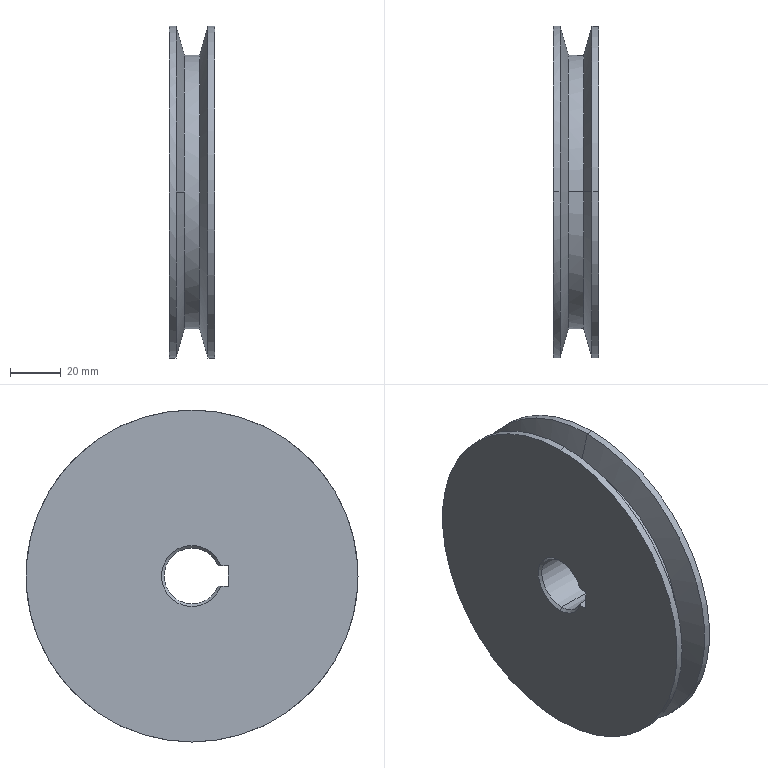Part | SolidWorks | features BaseBody 1 | 1 solid | 24 faces | box 18 x 130.5 x 130.5 mm | volume 193093 mm3 | cone 10 | cylinder 9 | plane 5 | commonest cylinder face diameters 130.5 x4 22 x3 107.6 x2
STEP:
#1=CARTESIAN_POINT('',(18.,0.,65.25));
#2=VERTEX_POINT('',#1);
#3=CARTESIAN_POINT('',(18.,0.,-65.25));
#4=VERTEX_POINT('',#3);
#5=CARTESIAN_POINT('',(18.,0.,0.));
#6=DIRECTION('',(-1.,0.,0.));
#7=DIRECTION('',(0.,0.,1.));
#8=AXIS2_PLACEMENT_3D('',#5,#6,#7);
#9=CIRCLE('',#8,65.25);
#10=EDGE_CURVE('',#2,#4,#9,.T.);
#11=ORIENTED_EDGE('',*,*,#10,.T.);
#12=CARTESIAN_POINT('',(15.289,0.,-65.25));
#13=VERTEX_POINT('',#12);
#14=CARTESIAN_POINT('',(0.,0.,-65.25));
#15=DIRECTION('',(-1.,0.,0.));
#16=VECTOR('',#15,1000.);
#17=LINE('',#14,#16);
#18=EDGE_CURVE('',#4,#13,#17,.T.);
#19=ORIENTED_EDGE('',*,*,#18,.T.);
#20=CARTESIAN_POINT('',(15.289,0.,65.25));
#21=VERTEX_POINT('',#20);
#22=CARTESIAN_POINT('',(15.289,0.,0.));
#23=DIRECTION('',(1.,0.,0.));
#24=DIRECTION('',(0.,0.,1.));
#25=AXIS2_PLACEMENT_3D('',#22,#23,#24);
#26=CIRCLE('',#25,65.25);
#27=EDGE_CURVE('',#13,#21,#26,.T.);
#28=ORIENTED_EDGE('',*,*,#27,.T.);
#29=CARTESIAN_POINT('',(0.,0.,65.25));
#30=DIRECTION('',(-1.,0.,0.));
#31=VECTOR('',#30,1000.);
#32=LINE('',#29,#31);
#33=EDGE_CURVE('',#2,#21,#32,.T.);
#34=ORIENTED_EDGE('',*,*,#33,.F.);
#35=EDGE_LOOP('',(#11,#19,#28,#34));
#36=FACE_OUTER_BOUND('',#35,.T.);
#37=CARTESIAN_POINT('',(0.,0.,0.));
#38=DIRECTION('',(-1.,0.,0.));
#39=DIRECTION('',(0.,0.,1.));
#40=AXIS2_PLACEMENT_3D('',#37,#38,#39);
#41=CYLINDRICAL_SURFACE('',#40,65.25);
#42=ADVANCED_FACE('',(#36),#41,.T.);
#43=CARTESIAN_POINT('',(17.,0.,11.));
#44=VERTEX_POINT('',#43);
#45=CARTESIAN_POINT('',(17.,-10.247,4.));
#46=VERTEX_POINT('',#45);
#47=CARTESIAN_POINT('',(17.,0.,0.));
#48=DIRECTION('',(1.,0.,0.));
#49=DIRECTION('',(0.,0.,-1.));
#50=AXIS2_PLACEMENT_3D('',#47,#48,#49);
#51=CIRCLE('',#50,11.);
#52=EDGE_CURVE('',#44,#46,#51,.T.);
#53=ORIENTED_EDGE('',*,*,#52,.F.);
#54=CARTESIAN_POINT('',(18.,0.,12.));
#55=VERTEX_POINT('',#54);
#56=CARTESIAN_POINT('',(18.,0.,12.));
#57=DIRECTION('',(0.7071,0.,0.7071));
#58=VECTOR('',#57,1000.);
#59=LINE('',#56,#58);
#60=EDGE_CURVE('',#44,#55,#59,.T.);
#61=ORIENTED_EDGE('',*,*,#60,.T.);
#62=CARTESIAN_POINT('',(18.,-11.314,4.));
#63=VERTEX_POINT('',#62);
#64=CARTESIAN_POINT('',(18.,0.,0.));
#65=DIRECTION('',(1.,0.,0.));
#66=DIRECTION('',(0.,0.,-1.));
#67=AXIS2_PLACEMENT_3D('',#64,#65,#66);
#68=CIRCLE('',#67,12.);
#69=EDGE_CURVE('',#55,#63,#68,.T.);
#70=ORIENTED_EDGE('',*,*,#69,.T.);
#71=CARTESIAN_POINT('',(18.,-11.314,4.));
#72=CARTESIAN_POINT('',(17.666,-10.959,4.));
#73=CARTESIAN_POINT('',(17.332,-10.604,4.));
#74=CARTESIAN_POINT('',(17.,-10.247,4.));
#75=B_SPLINE_CURVE_WITH_KNOTS('',3,(#71,#72,#73,#74),.UNSPECIFIED.,.F.,.F.,(4,4),(0.,0.001462),.UNSPECIFIED.);
#76=EDGE_CURVE('',#63,#46,#75,.T.);
#77=ORIENTED_EDGE('',*,*,#76,.T.);
#78=EDGE_LOOP('',(#53,#61,#70,#77));
#79=FACE_OUTER_BOUND('',#78,.T.);
#80=CARTESIAN_POINT('',(18.,0.,0.));
#81=DIRECTION('',(1.,0.,0.));
#82=DIRECTION('',(0.,0.,-1.));
#83=AXIS2_PLACEMENT_3D('',#80,#81,#82);
#84=CONICAL_SURFACE('',#83,12.,0.7854);
#85=ADVANCED_FACE('',(#79),#84,.F.);
#86=ORIENTED_EDGE('',*,*,#60,.F.);
#87=CARTESIAN_POINT('',(17.,0.,-11.));
#88=VERTEX_POINT('',#87);
#89=CARTESIAN_POINT('',(17.,0.,0.));
#90=DIRECTION('',(1.,0.,0.));
#91=DIRECTION('',(0.,0.,-1.));
#92=AXIS2_PLACEMENT_3D('',#89,#90,#91);
#93=CIRCLE('',#92,11.);
#94=EDGE_CURVE('',#88,#44,#93,.T.);
#95=ORIENTED_EDGE('',*,*,#94,.F.);
#96=CARTESIAN_POINT('',(18.,0.,-12.));
#97=VERTEX_POINT('',#96);
#98=CARTESIAN_POINT('',(18.,0.,-12.));
#99=DIRECTION('',(0.7071,0.,-0.7071));
#100=VECTOR('',#99,1000.);
#101=LINE('',#98,#100);
#102=EDGE_CURVE('',#88,#97,#101,.T.);
#103=ORIENTED_EDGE('',*,*,#102,.T.);
#104=CARTESIAN_POINT('',(18.,0.,0.));
#105=DIRECTION('',(1.,0.,0.));
#106=DIRECTION('',(0.,0.,-1.));
#107=AXIS2_PLACEMENT_3D('',#104,#105,#106);
#108=CIRCLE('',#107,12.);
#109=EDGE_CURVE('',#97,#55,#108,.T.);
#110=ORIENTED_EDGE('',*,*,#109,.T.);
#111=EDGE_LOOP('',(#86,#95,#103,#110));
#112=FACE_OUTER_BOUND('',#111,.T.);
#113=CARTESIAN_POINT('',(18.,0.,0.));
#114=DIRECTION('',(1.,0.,0.));
#115=DIRECTION('',(0.,0.,-1.));
#116=AXIS2_PLACEMENT_3D('',#113,#114,#115);
#117=CONICAL_SURFACE('',#116,12.,0.7854);
#118=ADVANCED_FACE('',(#112),#117,.F.);
#119=CARTESIAN_POINT('',(12.005,0.,-53.8));
#120=VERTEX_POINT('',#119);
#121=CARTESIAN_POINT('',(12.005,0.,53.8));
#122=VERTEX_POINT('',#121);
#123=CARTESIAN_POINT('',(12.005,0.,0.));
#124=DIRECTION('',(1.,0.,0.));
#125=DIRECTION('',(0.,0.,-1.));
#126=AXIS2_PLACEMENT_3D('',#123,#124,#125);
#127=CIRCLE('',#126,53.8);
#128=EDGE_CURVE('',#120,#122,#127,.T.);
#129=ORIENTED_EDGE('',*,*,#128,.T.);
#130=CARTESIAN_POINT('',(15.289,0.,65.25));
#131=DIRECTION('',(0.2756,0.,0.9613));
#132=VECTOR('',#131,1000.);
#133=LINE('',#130,#132);
#134=EDGE_CURVE('',#122,#21,#133,.T.);
#135=ORIENTED_EDGE('',*,*,#134,.T.);
#136=ORIENTED_EDGE('',*,*,#27,.F.);
#137=CARTESIAN_POINT('',(15.289,0.,-65.25));
#138=DIRECTION('',(0.2756,0.,-0.9613));
#139=VECTOR('',#138,1000.);
#140=LINE('',#137,#139);
#141=EDGE_CURVE('',#120,#13,#140,.T.);
#142=ORIENTED_EDGE('',*,*,#141,.F.);
#143=EDGE_LOOP('',(#129,#135,#136,#142));
#144=FACE_OUTER_BOUND('',#143,.T.);
#145=CARTESIAN_POINT('',(15.289,0.,0.));
#146=DIRECTION('',(1.,0.,0.));
#147=DIRECTION('',(0.,0.,-1.));
#148=AXIS2_PLACEMENT_3D('',#145,#146,#147);
#149=CONICAL_SURFACE('',#148,65.25,1.292);
#150=ADVANCED_FACE('',(#144),#149,.T.);
#151=CARTESIAN_POINT('',(17.,-10.247,-4.));
#152=VERTEX_POINT('',#151);
#153=CARTESIAN_POINT('',(17.,0.,0.));
#154=DIRECTION('',(1.,0.,0.));
#155=DIRECTION('',(0.,0.,-1.));
#156=AXIS2_PLACEMENT_3D('',#153,#154,#155);
#157=CIRCLE('',#156,11.);
#158=EDGE_CURVE('',#152,#88,#157,.T.);
#159=ORIENTED_EDGE('',*,*,#158,.T.);
#160=CARTESIAN_POINT('',(1.,0.,-11.));
#161=VERTEX_POINT('',#160);
#162=CARTESIAN_POINT('',(0.,0.,-11.));
#163=DIRECTION('',(-1.,0.,0.));
#164=VECTOR('',#163,1000.);
#165=LINE('',#162,#164);
#166=EDGE_CURVE('',#88,#161,#165,.T.);
#167=ORIENTED_EDGE('',*,*,#166,.T.);
#168=CARTESIAN_POINT('',(1.,-10.247,-4.));
#169=VERTEX_POINT('',#168);
#170=CARTESIAN_POINT('',(1.,0.,0.));
#171=DIRECTION('',(1.,0.,0.));
#172=DIRECTION('',(0.,0.,1.));
#173=AXIS2_PLACEMENT_3D('',#170,#171,#172);
#174=CIRCLE('',#173,11.);
#175=EDGE_CURVE('',#169,#161,#174,.T.);
#176=ORIENTED_EDGE('',*,*,#175,.F.);
#177=CARTESIAN_POINT('',(44.,-10.247,-4.));
#178=DIRECTION('',(1.,0.,0.));
#179=VECTOR('',#178,1000.);
#180=LINE('',#177,#179);
#181=EDGE_CURVE('',#169,#152,#180,.T.);
#182=ORIENTED_EDGE('',*,*,#181,.T.);
#183=EDGE_LOOP('',(#159,#167,#176,#182));
#184=FACE_OUTER_BOUND('',#183,.T.);
#185=CARTESIAN_POINT('',(0.,0.,0.));
#186=DIRECTION('',(-1.,0.,0.));
#187=DIRECTION('',(0.,0.,1.));
#188=AXIS2_PLACEMENT_3D('',#185,#186,#187);
#189=CYLINDRICAL_SURFACE('',#188,11.);
#190=ADVANCED_FACE('',(#184),#189,.F.);
#191=ORIENTED_EDGE('',*,*,#166,.F.);
#192=ORIENTED_EDGE('',*,*,#94,.T.);
#193=CARTESIAN_POINT('',(1.,0.,11.));
#194=VERTEX_POINT('',#193);
#195=CARTESIAN_POINT('',(0.,0.,11.));
#196=DIRECTION('',(-1.,0.,0.));
#197=VECTOR('',#196,1000.);
#198=LINE('',#195,#197);
#199=EDGE_CURVE('',#44,#194,#198,.T.);
#200=ORIENTED_EDGE('',*,*,#199,.T.);
#201=CARTESIAN_POINT('',(1.,0.,0.));
#202=DIRECTION('',(1.,0.,0.));
#203=DIRECTION('',(0.,0.,1.));
#204=AXIS2_PLACEMENT_3D('',#201,#202,#203);
#205=CIRCLE('',#204,11.);
#206=EDGE_CURVE('',#161,#194,#205,.T.);
#207=ORIENTED_EDGE('',*,*,#206,.F.);
#208=EDGE_LOOP('',(#191,#192,#200,#207));
#209=FACE_OUTER_BOUND('',#208,.T.);
#210=CARTESIAN_POINT('',(0.,0.,0.));
#211=DIRECTION('',(-1.,0.,0.));
#212=DIRECTION('',(0.,0.,1.));
#213=AXIS2_PLACEMENT_3D('',#210,#211,#212);
#214=CYLINDRICAL_SURFACE('',#213,11.);
#215=ADVANCED_FACE('',(#209),#214,.F.);
#216=ORIENTED_EDGE('',*,*,#128,.F.);
#217=CARTESIAN_POINT('',(5.995,0.,-53.8));
#218=VERTEX_POINT('',#217);
#219=CARTESIAN_POINT('',(0.,0.,-53.8));
#220=DIRECTION('',(-1.,0.,0.));
#221=VECTOR('',#220,1000.);
#222=LINE('',#219,#221);
#223=EDGE_CURVE('',#120,#218,#222,.T.);
#224=ORIENTED_EDGE('',*,*,#223,.T.);
#225=CARTESIAN_POINT('',(5.995,53.8,0.));
#226=VERTEX_POINT('',#225);
#227=CARTESIAN_POINT('',(5.995,0.,0.));
#228=DIRECTION('',(1.,0.,0.));
#229=DIRECTION('',(0.,0.,1.));
#230=AXIS2_PLACEMENT_3D('',#227,#228,#229);
#231=CIRCLE('',#230,53.8);
#232=EDGE_CURVE('',#218,#226,#231,.T.);
#233=ORIENTED_EDGE('',*,*,#232,.T.);
#234=CARTESIAN_POINT('',(5.995,0.,53.8));
#235=VERTEX_POINT('',#234);
#236=CARTESIAN_POINT('',(5.995,0.,0.));
#237=DIRECTION('',(1.,0.,0.));
#238=DIRECTION('',(0.,0.,1.));
#239=AXIS2_PLACEMENT_3D('',#236,#237,#238);
#240=CIRCLE('',#239,53.8);
#241=EDGE_CURVE('',#226,#235,#240,.T.);
#242=ORIENTED_EDGE('',*,*,#241,.T.);
#243=CARTESIAN_POINT('',(0.,0.,53.8));
#244=DIRECTION('',(-1.,0.,0.));
#245=VECTOR('',#244,1000.);
#246=LINE('',#243,#245);
#247=EDGE_CURVE('',#122,#235,#246,.T.);
#248=ORIENTED_EDGE('',*,*,#247,.F.);
#249=EDGE_LOOP('',(#216,#224,#233,#242,#248));
#250=FACE_OUTER_BOUND('',#249,.T.);
#251=CARTESIAN_POINT('',(0.,0.,0.));
#252=DIRECTION('',(-1.,0.,0.));
#253=DIRECTION('',(0.,0.,1.));
#254=AXIS2_PLACEMENT_3D('',#251,#252,#253);
#255=CYLINDRICAL_SURFACE('',#254,53.8);
#256=ADVANCED_FACE('',(#250),#255,.T.);
#257=CARTESIAN_POINT('',(2.711,65.25,0.));
#258=VERTEX_POINT('',#257);
#259=CARTESIAN_POINT('',(2.711,0.,-65.25));
#260=VERTEX_POINT('',#259);
#261=CARTESIAN_POINT('',(2.711,0.,0.));
#262=DIRECTION('',(-1.,0.,0.));
#263=DIRECTION('',(0.,0.,1.));
#264=AXIS2_PLACEMENT_3D('',#261,#262,#263);
#265=CIRCLE('',#264,65.25);
#266=EDGE_CURVE('',#258,#260,#265,.T.);
#267=ORIENTED_EDGE('',*,*,#266,.T.);
#268=CARTESIAN_POINT('',(0.,0.,-65.25));
#269=VERTEX_POINT('',#268);
#270=CARTESIAN_POINT('',(0.,0.,-65.25));
#271=DIRECTION('',(-1.,0.,0.));
#272=VECTOR('',#271,1000.);
#273=LINE('',#270,#272);
#274=EDGE_CURVE('',#260,#269,#273,.T.);
#275=ORIENTED_EDGE('',*,*,#274,.T.);
#276=CARTESIAN_POINT('',(0.,0.,65.25));
#277=VERTEX_POINT('',#276);
#278=CARTESIAN_POINT('',(0.,0.,0.));
#279=DIRECTION('',(1.,0.,0.));
#280=DIRECTION('',(0.,0.,1.));
#281=AXIS2_PLACEMENT_3D('',#278,#279,#280);
#282=CIRCLE('',#281,65.25);
#283=EDGE_CURVE('',#269,#277,#282,.T.);
#284=ORIENTED_EDGE('',*,*,#283,.T.);
#285=CARTESIAN_POINT('',(2.711,0.,65.25));
#286=VERTEX_POINT('',#285);
#287=CARTESIAN_POINT('',(0.,0.,65.25));
#288=DIRECTION('',(-1.,0.,0.));
#289=VECTOR('',#288,1000.);
#290=LINE('',#287,#289);
#291=EDGE_CURVE('',#286,#277,#290,.T.);
#292=ORIENTED_EDGE('',*,*,#291,.F.);
#293=CARTESIAN_POINT('',(2.711,0.,0.));
#294=DIRECTION('',(-1.,0.,0.));
#295=DIRECTION('',(0.,0.,1.));
#296=AXIS2_PLACEMENT_3D('',#293,#294,#295);
#297=CIRCLE('',#296,65.25);
#298=EDGE_CURVE('',#286,#258,#297,.T.);
#299=ORIENTED_EDGE('',*,*,#298,.T.);
#300=EDGE_LOOP('',(#267,#275,#284,#292,#299));
#301=FACE_OUTER_BOUND('',#300,.T.);
#302=CARTESIAN_POINT('',(0.,0.,0.));
#303=DIRECTION('',(-1.,0.,0.));
#304=DIRECTION('',(0.,0.,1.));
#305=AXIS2_PLACEMENT_3D('',#302,#303,#304);
#306=CYLINDRICAL_SURFACE('',#305,65.25);
#307=ADVANCED_FACE('',(#301),#306,.T.);
#308=ORIENTED_EDGE('',*,*,#175,.T.);
#309=CARTESIAN_POINT('',(0.,0.,-12.));
#310=VERTEX_POINT('',#309);
#311=CARTESIAN_POINT('',(0.,0.,-12.));
#312=DIRECTION('',(-0.7071,0.,-0.7071));
#313=VECTOR('',#312,1000.);
#314=LINE('',#311,#313);
#315=EDGE_CURVE('',#161,#310,#314,.T.);
#316=ORIENTED_EDGE('',*,*,#315,.T.);
#317=CARTESIAN_POINT('',(0.,-11.314,-4.));
#318=VERTEX_POINT('',#317);
#319=CARTESIAN_POINT('',(0.,0.,0.));
#320=DIRECTION('',(-1.,0.,0.));
#321=DIRECTION('',(0.,0.,1.));
#322=AXIS2_PLACEMENT_3D('',#319,#320,#321);
#323=CIRCLE('',#322,12.);
#324=EDGE_CURVE('',#310,#318,#323,.T.);
#325=ORIENTED_EDGE('',*,*,#324,.T.);
#326=CARTESIAN_POINT('',(1.,-10.247,-4.));
#327=CARTESIAN_POINT('',(0.6832,-10.587,-4.));
#328=CARTESIAN_POINT('',(0.3498,-10.943,-4.));
#329=CARTESIAN_POINT('',(0.,-11.314,-4.));
#330=B_SPLINE_CURVE_WITH_KNOTS('',3,(#326,#327,#328,#329),.UNSPECIFIED.,.F.,.F.,(4,4),(0.,1.),.UNSPECIFIED.);
#331=EDGE_CURVE('',#169,#318,#330,.T.);
#332=ORIENTED_EDGE('',*,*,#331,.F.);
#333=EDGE_LOOP('',(#308,#316,#325,#332));
#334=FACE_OUTER_BOUND('',#333,.T.);
#335=CARTESIAN_POINT('',(0.,0.,0.));
#336=DIRECTION('',(-1.,0.,0.));
#337=DIRECTION('',(0.,0.,1.));
#338=AXIS2_PLACEMENT_3D('',#335,#336,#337);
#339=CONICAL_SURFACE('',#338,12.,0.7854);
#340=ADVANCED_FACE('',(#334),#339,.F.);
#341=ORIENTED_EDGE('',*,*,#315,.F.);
#342=ORIENTED_EDGE('',*,*,#206,.T.);
#343=CARTESIAN_POINT('',(0.,0.,12.));
#344=VERTEX_POINT('',#343);
#345=CARTESIAN_POINT('',(0.,0.,12.));
#346=DIRECTION('',(-0.7071,0.,0.7071));
#347=VECTOR('',#346,1000.);
#348=LINE('',#345,#347);
#349=EDGE_CURVE('',#194,#344,#348,.T.);
#350=ORIENTED_EDGE('',*,*,#349,.T.);
#351=CARTESIAN_POINT('',(0.,0.,0.));
#352=DIRECTION('',(-1.,0.,0.));
#353=DIRECTION('',(0.,0.,1.));
#354=AXIS2_PLACEMENT_3D('',#351,#352,#353);
#355=CIRCLE('',#354,12.);
#356=EDGE_CURVE('',#344,#310,#355,.T.);
#357=ORIENTED_EDGE('',*,*,#356,.T.);
#358=EDGE_LOOP('',(#341,#342,#350,#357));
#359=FACE_OUTER_BOUND('',#358,.T.);
#360=CARTESIAN_POINT('',(0.,0.,0.));
#361=DIRECTION('',(-1.,0.,0.));
#362=DIRECTION('',(0.,0.,1.));
#363=AXIS2_PLACEMENT_3D('',#360,#361,#362);
#364=CONICAL_SURFACE('',#363,12.,0.7854);
#365=ADVANCED_FACE('',(#359),#364,.F.);
#366=ORIENTED_EDGE('',*,*,#241,.F.);
#367=CARTESIAN_POINT('',(2.711,65.25,0.));
#368=DIRECTION('',(-0.2756,0.9613,0.));
#369=VECTOR('',#368,1000.);
#370=LINE('',#367,#369);
#371=EDGE_CURVE('',#226,#258,#370,.T.);
#372=ORIENTED_EDGE('',*,*,#371,.T.);
#373=ORIENTED_EDGE('',*,*,#298,.F.);
#374=CARTESIAN_POINT('',(2.711,-65.25,0.));
#375=VERTEX_POINT('',#374);
#376=CARTESIAN_POINT('',(2.711,0.,0.));
#377=DIRECTION('',(-1.,0.,0.));
#378=DIRECTION('',(0.,0.,1.));
#379=AXIS2_PLACEMENT_3D('',#376,#377,#378);
#380=CIRCLE('',#379,65.25);
#381=EDGE_CURVE('',#375,#286,#380,.T.);
#382=ORIENTED_EDGE('',*,*,#381,.F.);
#383=CARTESIAN_POINT('',(5.995,-53.8,0.));
#384=VERTEX_POINT('',#383);
#385=CARTESIAN_POINT('',(2.711,-65.25,0.));
#386=DIRECTION('',(-0.2756,-0.9613,0.));
#387=VECTOR('',#386,1000.);
#388=LINE('',#385,#387);
#389=EDGE_CURVE('',#384,#375,#388,.T.);
#390=ORIENTED_EDGE('',*,*,#389,.F.);
#391=CARTESIAN_POINT('',(5.995,0.,0.));
#392=DIRECTION('',(1.,0.,0.));
#393=DIRECTION('',(0.,0.,1.));
#394=AXIS2_PLACEMENT_3D('',#391,#392,#393);
#395=CIRCLE('',#394,53.8);
#396=EDGE_CURVE('',#235,#384,#395,.T.);
#397=ORIENTED_EDGE('',*,*,#396,.F.);
#398=EDGE_LOOP('',(#366,#372,#373,#382,#390,#397));
#399=FACE_OUTER_BOUND('',#398,.T.);
#400=CARTESIAN_POINT('',(2.711,0.,0.));
#401=DIRECTION('',(-1.,0.,0.));
#402=DIRECTION('',(0.,-1.,0.));
#403=AXIS2_PLACEMENT_3D('',#400,#401,#402);
#404=CONICAL_SURFACE('',#403,65.25,1.292);
#405=ADVANCED_FACE('',(#399),#404,.T.);
#406=ORIENTED_EDGE('',*,*,#10,.F.);
#407=CARTESIAN_POINT('',(18.,0.,0.));
#408=DIRECTION('',(-1.,0.,0.));
#409=DIRECTION('',(0.,0.,1.));
#410=AXIS2_PLACEMENT_3D('',#407,#408,#409);
#411=CIRCLE('',#410,65.25);
#412=EDGE_CURVE('',#4,#2,#411,.T.);
#413=ORIENTED_EDGE('',*,*,#412,.F.);
#414=EDGE_LOOP('',(#406,#413));
#415=FACE_OUTER_BOUND('',#414,.T.);
#416=CARTESIAN_POINT('',(18.,-14.3,4.));
#417=VERTEX_POINT('',#416);
#418=CARTESIAN_POINT('',(18.,65.25,4.));
#419=DIRECTION('',(0.,-1.,0.));
#420=VECTOR('',#419,1000.);
#421=LINE('',#418,#420);
#422=EDGE_CURVE('',#63,#417,#421,.T.);
#423=ORIENTED_EDGE('',*,*,#422,.F.);
#424=ORIENTED_EDGE('',*,*,#69,.F.);
#425=ORIENTED_EDGE('',*,*,#109,.F.);
#426=CARTESIAN_POINT('',(18.,-11.314,-4.));
#427=VERTEX_POINT('',#426);
#428=CARTESIAN_POINT('',(18.,0.,0.));
#429=DIRECTION('',(1.,0.,0.));
#430=DIRECTION('',(0.,0.,-1.));
#431=AXIS2_PLACEMENT_3D('',#428,#429,#430);
#432=CIRCLE('',#431,12.);
#433=EDGE_CURVE('',#427,#97,#432,.T.);
#434=ORIENTED_EDGE('',*,*,#433,.F.);
#435=CARTESIAN_POINT('',(18.,-14.3,-4.));
#436=VERTEX_POINT('',#435);
#437=CARTESIAN_POINT('',(18.,65.25,-4.));
#438=DIRECTION('',(0.,1.,0.));
#439=VECTOR('',#438,1000.);
#440=LINE('',#437,#439);
#441=EDGE_CURVE('',#436,#427,#440,.T.);
#442=ORIENTED_EDGE('',*,*,#441,.F.);
#443=CARTESIAN_POINT('',(18.,-14.3,0.));
#444=DIRECTION('',(0.,0.,-1.));
#445=VECTOR('',#444,1000.);
#446=LINE('',#443,#445);
#447=EDGE_CURVE('',#417,#436,#446,.T.);
#448=ORIENTED_EDGE('',*,*,#447,.F.);
#449=EDGE_LOOP('',(#423,#424,#425,#434,#442,#448));
#450=FACE_BOUND('',#449,.T.);
#451=CARTESIAN_POINT('',(18.,65.25,0.));
#452=DIRECTION('',(-1.,0.,0.));
#453=DIRECTION('',(0.,0.,1.));
#454=AXIS2_PLACEMENT_3D('',#451,#452,#453);
#455=PLANE('',#454);
#456=ADVANCED_FACE('',(#415,#450),#455,.F.);
#457=ORIENTED_EDGE('',*,*,#18,.F.);
#458=ORIENTED_EDGE('',*,*,#412,.T.);
#459=ORIENTED_EDGE('',*,*,#33,.T.);
#460=CARTESIAN_POINT('',(15.289,0.,0.));
#461=DIRECTION('',(1.,0.,0.));
#462=DIRECTION('',(0.,0.,1.));
#463=AXIS2_PLACEMENT_3D('',#460,#461,#462);
#464=CIRCLE('',#463,65.25);
#465=EDGE_CURVE('',#21,#13,#464,.T.);
#466=ORIENTED_EDGE('',*,*,#465,.T.);
#467=EDGE_LOOP('',(#457,#458,#459,#466));
#468=FACE_OUTER_BOUND('',#467,.T.);
#469=CARTESIAN_POINT('',(0.,0.,0.));
#470=DIRECTION('',(-1.,0.,0.));
#471=DIRECTION('',(0.,0.,1.));
#472=AXIS2_PLACEMENT_3D('',#469,#470,#471);
#473=CYLINDRICAL_SURFACE('',#472,65.25);
#474=ADVANCED_FACE('',(#468),#473,.T.);
#475=CARTESIAN_POINT('',(0.,-14.3,4.));
#476=VERTEX_POINT('',#475);
#477=CARTESIAN_POINT('',(0.,-14.3,-4.));
#478=VERTEX_POINT('',#477);
#479=CARTESIAN_POINT('',(0.,-14.3,-4.));
#480=DIRECTION('',(0.,0.,-1.));
#481=VECTOR('',#480,1000.);
#482=LINE('',#479,#481);
#483=EDGE_CURVE('',#476,#478,#482,.T.);
#484=ORIENTED_EDGE('',*,*,#483,.F.);
#485=CARTESIAN_POINT('',(44.,-14.3,4.));
#486=DIRECTION('',(-1.,0.,0.));
#487=VECTOR('',#486,1000.);
#488=LINE('',#485,#487);
#489=EDGE_CURVE('',#417,#476,#488,.T.);
#490=ORIENTED_EDGE('',*,*,#489,.F.);
#491=ORIENTED_EDGE('',*,*,#447,.T.);
#492=CARTESIAN_POINT('',(44.,-14.3,-4.));
#493=DIRECTION('',(1.,0.,0.));
#494=VECTOR('',#493,1000.);
#495=LINE('',#492,#494);
#496=EDGE_CURVE('',#478,#436,#495,.T.);
#497=ORIENTED_EDGE('',*,*,#496,.F.);
#498=EDGE_LOOP('',(#484,#490,#491,#497));
#499=FACE_OUTER_BOUND('',#498,.T.);
#500=CARTESIAN_POINT('',(44.,-14.3,-4.));
#501=DIRECTION('',(0.,-1.,0.));
#502=DIRECTION('',(0.,0.,-1.));
#503=AXIS2_PLACEMENT_3D('',#500,#501,#502);
#504=PLANE('',#503);
#505=ADVANCED_FACE('',(#499),#504,.F.);
#506=CARTESIAN_POINT('',(0.,-11.314,4.));
#507=VERTEX_POINT('',#506);
#508=CARTESIAN_POINT('',(0.,-14.3,4.));
#509=DIRECTION('',(0.,-1.,0.));
#510=VECTOR('',#509,1000.);
#511=LINE('',#508,#510);
#512=EDGE_CURVE('',#507,#476,#511,.T.);
#513=ORIENTED_EDGE('',*,*,#512,.F.);
#514=CARTESIAN_POINT('',(1.,-10.247,4.));
#515=VERTEX_POINT('',#514);
#516=CARTESIAN_POINT('',(0.,-11.314,4.));
#517=CARTESIAN_POINT('',(0.3498,-10.943,4.));
#518=CARTESIAN_POINT('',(0.6832,-10.587,4.));
#519=CARTESIAN_POINT('',(1.,-10.247,4.));
#520=B_SPLINE_CURVE_WITH_KNOTS('',3,(#516,#517,#518,#519),.UNSPECIFIED.,.F.,.F.,(4,4),(0.,1.),.UNSPECIFIED.);
#521=EDGE_CURVE('',#507,#515,#520,.T.);
#522=ORIENTED_EDGE('',*,*,#521,.T.);
#523=CARTESIAN_POINT('',(44.,-10.247,4.));
#524=DIRECTION('',(-1.,0.,0.));
#525=VECTOR('',#524,1000.);
#526=LINE('',#523,#525);
#527=EDGE_CURVE('',#46,#515,#526,.T.);
#528=ORIENTED_EDGE('',*,*,#527,.F.);
#529=ORIENTED_EDGE('',*,*,#76,.F.);
#530=ORIENTED_EDGE('',*,*,#422,.T.);
#531=ORIENTED_EDGE('',*,*,#489,.T.);
#532=EDGE_LOOP('',(#513,#522,#528,#529,#530,#531));
#533=FACE_OUTER_BOUND('',#532,.T.);
#534=CARTESIAN_POINT('',(44.,-14.3,4.));
#535=DIRECTION('',(0.,0.,1.));
#536=DIRECTION('',(1.,0.,0.));
#537=AXIS2_PLACEMENT_3D('',#534,#535,#536);
#538=PLANE('',#537);
#539=ADVANCED_FACE('',(#533),#538,.F.);
#540=ORIENTED_EDGE('',*,*,#102,.F.);
#541=ORIENTED_EDGE('',*,*,#158,.F.);
#542=CARTESIAN_POINT('',(18.,-11.314,-4.));
#543=CARTESIAN_POINT('',(17.65,-10.943,-4.));
#544=CARTESIAN_POINT('',(17.317,-10.587,-4.));
#545=CARTESIAN_POINT('',(17.,-10.247,-4.));
#546=B_SPLINE_CURVE_WITH_KNOTS('',3,(#542,#543,#544,#545),.UNSPECIFIED.,.F.,.F.,(4,4),(0.,1.),.UNSPECIFIED.);
#547=EDGE_CURVE('',#427,#152,#546,.T.);
#548=ORIENTED_EDGE('',*,*,#547,.F.);
#549=ORIENTED_EDGE('',*,*,#433,.T.);
#550=EDGE_LOOP('',(#540,#541,#548,#549));
#551=FACE_OUTER_BOUND('',#550,.T.);
#552=CARTESIAN_POINT('',(18.,0.,0.));
#553=DIRECTION('',(1.,0.,0.));
#554=DIRECTION('',(0.,0.,-1.));
#555=AXIS2_PLACEMENT_3D('',#552,#553,#554);
#556=CONICAL_SURFACE('',#555,12.,0.7854);
#557=ADVANCED_FACE('',(#551),#556,.F.);
#558=ORIENTED_EDGE('',*,*,#181,.F.);
#559=ORIENTED_EDGE('',*,*,#331,.T.);
#560=CARTESIAN_POINT('',(0.,-14.3,-4.));
#561=DIRECTION('',(0.,1.,0.));
#562=VECTOR('',#561,1000.);
#563=LINE('',#560,#562);
#564=EDGE_CURVE('',#478,#318,#563,.T.);
#565=ORIENTED_EDGE('',*,*,#564,.F.);
#566=ORIENTED_EDGE('',*,*,#496,.T.);
#567=ORIENTED_EDGE('',*,*,#441,.T.);
#568=ORIENTED_EDGE('',*,*,#547,.T.);
#569=EDGE_LOOP('',(#558,#559,#565,#566,#567,#568));
#570=FACE_OUTER_BOUND('',#569,.T.);
#571=CARTESIAN_POINT('',(44.,-14.3,-4.));
#572=DIRECTION('',(0.,0.,-1.));
#573=DIRECTION('',(-1.,0.,0.));
#574=AXIS2_PLACEMENT_3D('',#571,#572,#573);
#575=PLANE('',#574);
#576=ADVANCED_FACE('',(#570),#575,.F.);
#577=ORIENTED_EDGE('',*,*,#134,.F.);
#578=CARTESIAN_POINT('',(12.005,0.,0.));
#579=DIRECTION('',(1.,0.,0.));
#580=DIRECTION('',(0.,0.,-1.));
#581=AXIS2_PLACEMENT_3D('',#578,#579,#580);
#582=CIRCLE('',#581,53.8);
#583=EDGE_CURVE('',#122,#120,#582,.T.);
#584=ORIENTED_EDGE('',*,*,#583,.T.);
#585=ORIENTED_EDGE('',*,*,#141,.T.);
#586=ORIENTED_EDGE('',*,*,#465,.F.);
#587=EDGE_LOOP('',(#577,#584,#585,#586));
#588=FACE_OUTER_BOUND('',#587,.T.);
#589=CARTESIAN_POINT('',(15.289,0.,0.));
#590=DIRECTION('',(1.,0.,0.));
#591=DIRECTION('',(0.,0.,-1.));
#592=AXIS2_PLACEMENT_3D('',#589,#590,#591);
#593=CONICAL_SURFACE('',#592,65.25,1.292);
#594=ADVANCED_FACE('',(#588),#593,.T.);
#595=CARTESIAN_POINT('',(0.,0.,0.));
#596=DIRECTION('',(1.,0.,0.));
#597=DIRECTION('',(0.,0.,1.));
#598=AXIS2_PLACEMENT_3D('',#595,#596,#597);
#599=CIRCLE('',#598,65.25);
#600=EDGE_CURVE('',#277,#269,#599,.T.);
#601=ORIENTED_EDGE('',*,*,#600,.F.);
#602=ORIENTED_EDGE('',*,*,#283,.F.);
#603=EDGE_LOOP('',(#601,#602));
#604=FACE_OUTER_BOUND('',#603,.T.);
#605=CARTESIAN_POINT('',(0.,0.,0.));
#606=DIRECTION('',(-1.,0.,0.));
#607=DIRECTION('',(0.,0.,1.));
#608=AXIS2_PLACEMENT_3D('',#605,#606,#607);
#609=CIRCLE('',#608,12.);
#610=EDGE_CURVE('',#507,#344,#609,.T.);
#611=ORIENTED_EDGE('',*,*,#610,.F.);
#612=ORIENTED_EDGE('',*,*,#512,.T.);
#613=ORIENTED_EDGE('',*,*,#483,.T.);
#614=ORIENTED_EDGE('',*,*,#564,.T.);
#615=ORIENTED_EDGE('',*,*,#324,.F.);
#616=ORIENTED_EDGE('',*,*,#356,.F.);
#617=EDGE_LOOP('',(#611,#612,#613,#614,#615,#616));
#618=FACE_BOUND('',#617,.T.);
#619=CARTESIAN_POINT('',(0.,11.,0.));
#620=DIRECTION('',(1.,0.,0.));
#621=DIRECTION('',(0.,0.,-1.));
#622=AXIS2_PLACEMENT_3D('',#619,#620,#621);
#623=PLANE('',#622);
#624=ADVANCED_FACE('',(#604,#618),#623,.F.);
#625=ORIENTED_EDGE('',*,*,#199,.F.);
#626=ORIENTED_EDGE('',*,*,#52,.T.);
#627=ORIENTED_EDGE('',*,*,#527,.T.);
#628=CARTESIAN_POINT('',(1.,0.,0.));
#629=DIRECTION('',(1.,0.,0.));
#630=DIRECTION('',(0.,0.,1.));
#631=AXIS2_PLACEMENT_3D('',#628,#629,#630);
#632=CIRCLE('',#631,11.);
#633=EDGE_CURVE('',#194,#515,#632,.T.);
#634=ORIENTED_EDGE('',*,*,#633,.F.);
#635=EDGE_LOOP('',(#625,#626,#627,#634));
#636=FACE_OUTER_BOUND('',#635,.T.);
#637=CARTESIAN_POINT('',(0.,0.,0.));
#638=DIRECTION('',(-1.,0.,0.));
#639=DIRECTION('',(0.,0.,1.));
#640=AXIS2_PLACEMENT_3D('',#637,#638,#639);
#641=CYLINDRICAL_SURFACE('',#640,11.);
#642=ADVANCED_FACE('',(#636),#641,.F.);
#643=ORIENTED_EDGE('',*,*,#223,.F.);
#644=ORIENTED_EDGE('',*,*,#583,.F.);
#645=ORIENTED_EDGE('',*,*,#247,.T.);
#646=ORIENTED_EDGE('',*,*,#396,.T.);
#647=CARTESIAN_POINT('',(5.995,0.,0.));
#648=DIRECTION('',(1.,0.,0.));
#649=DIRECTION('',(0.,0.,1.));
#650=AXIS2_PLACEMENT_3D('',#647,#648,#649);
#651=CIRCLE('',#650,53.8);
#652=EDGE_CURVE('',#384,#218,#651,.T.);
#653=ORIENTED_EDGE('',*,*,#652,.T.);
#654=EDGE_LOOP('',(#643,#644,#645,#646,#653));
#655=FACE_OUTER_BOUND('',#654,.T.);
#656=CARTESIAN_POINT('',(0.,0.,0.));
#657=DIRECTION('',(-1.,0.,0.));
#658=DIRECTION('',(0.,0.,1.));
#659=AXIS2_PLACEMENT_3D('',#656,#657,#658);
#660=CYLINDRICAL_SURFACE('',#659,53.8);
#661=ADVANCED_FACE('',(#655),#660,.T.);
#662=ORIENTED_EDGE('',*,*,#274,.F.);
#663=CARTESIAN_POINT('',(2.711,0.,0.));
#664=DIRECTION('',(-1.,0.,0.));
#665=DIRECTION('',(0.,0.,1.));
#666=AXIS2_PLACEMENT_3D('',#663,#664,#665);
#667=CIRCLE('',#666,65.25);
#668=EDGE_CURVE('',#260,#375,#667,.T.);
#669=ORIENTED_EDGE('',*,*,#668,.T.);
#670=ORIENTED_EDGE('',*,*,#381,.T.);
#671=ORIENTED_EDGE('',*,*,#291,.T.);
#672=ORIENTED_EDGE('',*,*,#600,.T.);
#673=EDGE_LOOP('',(#662,#669,#670,#671,#672));
#674=FACE_OUTER_BOUND('',#673,.T.);
#675=CARTESIAN_POINT('',(0.,0.,0.));
#676=DIRECTION('',(-1.,0.,0.));
#677=DIRECTION('',(0.,0.,1.));
#678=AXIS2_PLACEMENT_3D('',#675,#676,#677);
#679=CYLINDRICAL_SURFACE('',#678,65.25);
#680=ADVANCED_FACE('',(#674),#679,.T.);
#681=ORIENTED_EDGE('',*,*,#349,.F.);
#682=ORIENTED_EDGE('',*,*,#633,.T.);
#683=ORIENTED_EDGE('',*,*,#521,.F.);
#684=ORIENTED_EDGE('',*,*,#610,.T.);
#685=EDGE_LOOP('',(#681,#682,#683,#684));
#686=FACE_OUTER_BOUND('',#685,.T.);
#687=CARTESIAN_POINT('',(0.,0.,0.));
#688=DIRECTION('',(-1.,0.,0.));
#689=DIRECTION('',(0.,0.,1.));
#690=AXIS2_PLACEMENT_3D('',#687,#688,#689);
#691=CONICAL_SURFACE('',#690,12.,0.7854);
#692=ADVANCED_FACE('',(#686),#691,.F.);
#693=ORIENTED_EDGE('',*,*,#371,.F.);
#694=ORIENTED_EDGE('',*,*,#232,.F.);
#695=ORIENTED_EDGE('',*,*,#652,.F.);
#696=ORIENTED_EDGE('',*,*,#389,.T.);
#697=ORIENTED_EDGE('',*,*,#668,.F.);
#698=ORIENTED_EDGE('',*,*,#266,.F.);
#699=EDGE_LOOP('',(#693,#694,#695,#696,#697,#698));
#700=FACE_OUTER_BOUND('',#699,.T.);
#701=CARTESIAN_POINT('',(2.711,0.,0.));
#702=DIRECTION('',(-1.,0.,0.));
#703=DIRECTION('',(0.,-1.,0.));
#704=AXIS2_PLACEMENT_3D('',#701,#702,#703);
#705=CONICAL_SURFACE('',#704,65.25,1.292);
#706=ADVANCED_FACE('',(#700),#705,.T.);
#707=CLOSED_SHELL('',(#42,#85,#118,#150,#190,#215,#256,#307,#340,#365,#405,#456,#474,#505,#539,#557,#576,#594,#624,#642,#661,#680,#692,#706));
#708=MANIFOLD_SOLID_BREP('',#707);
#709=CARTESIAN_POINT('',(0.,0.,0.));
#710=DIRECTION('',(0.,0.,1.));
#711=DIRECTION('',(1.,0.,0.));
#712=AXIS2_PLACEMENT_3D('',#709,#710,#711);
#713=(LENGTH_UNIT()NAMED_UNIT(*)SI_UNIT(.MILLI.,.METRE.));
#714=UNCERTAINTY_MEASURE_WITH_UNIT(LENGTH_MEASURE(0.00001),#713,'','');
#715=(NAMED_UNIT(*)PLANE_ANGLE_UNIT()SI_UNIT($,.RADIAN.));
#716=(NAMED_UNIT(*)SI_UNIT($,.STERADIAN.)SOLID_ANGLE_UNIT());
#717=(GEOMETRIC_REPRESENTATION_CONTEXT(3)GLOBAL_UNCERTAINTY_ASSIGNED_CONTEXT((#714))GLOBAL_UNIT_ASSIGNED_CONTEXT((#713,#715,#716))REPRESENTATION_CONTEXT('',''));
#718=ADVANCED_BREP_SHAPE_REPRESENTATION('',(#708,#712),#717);